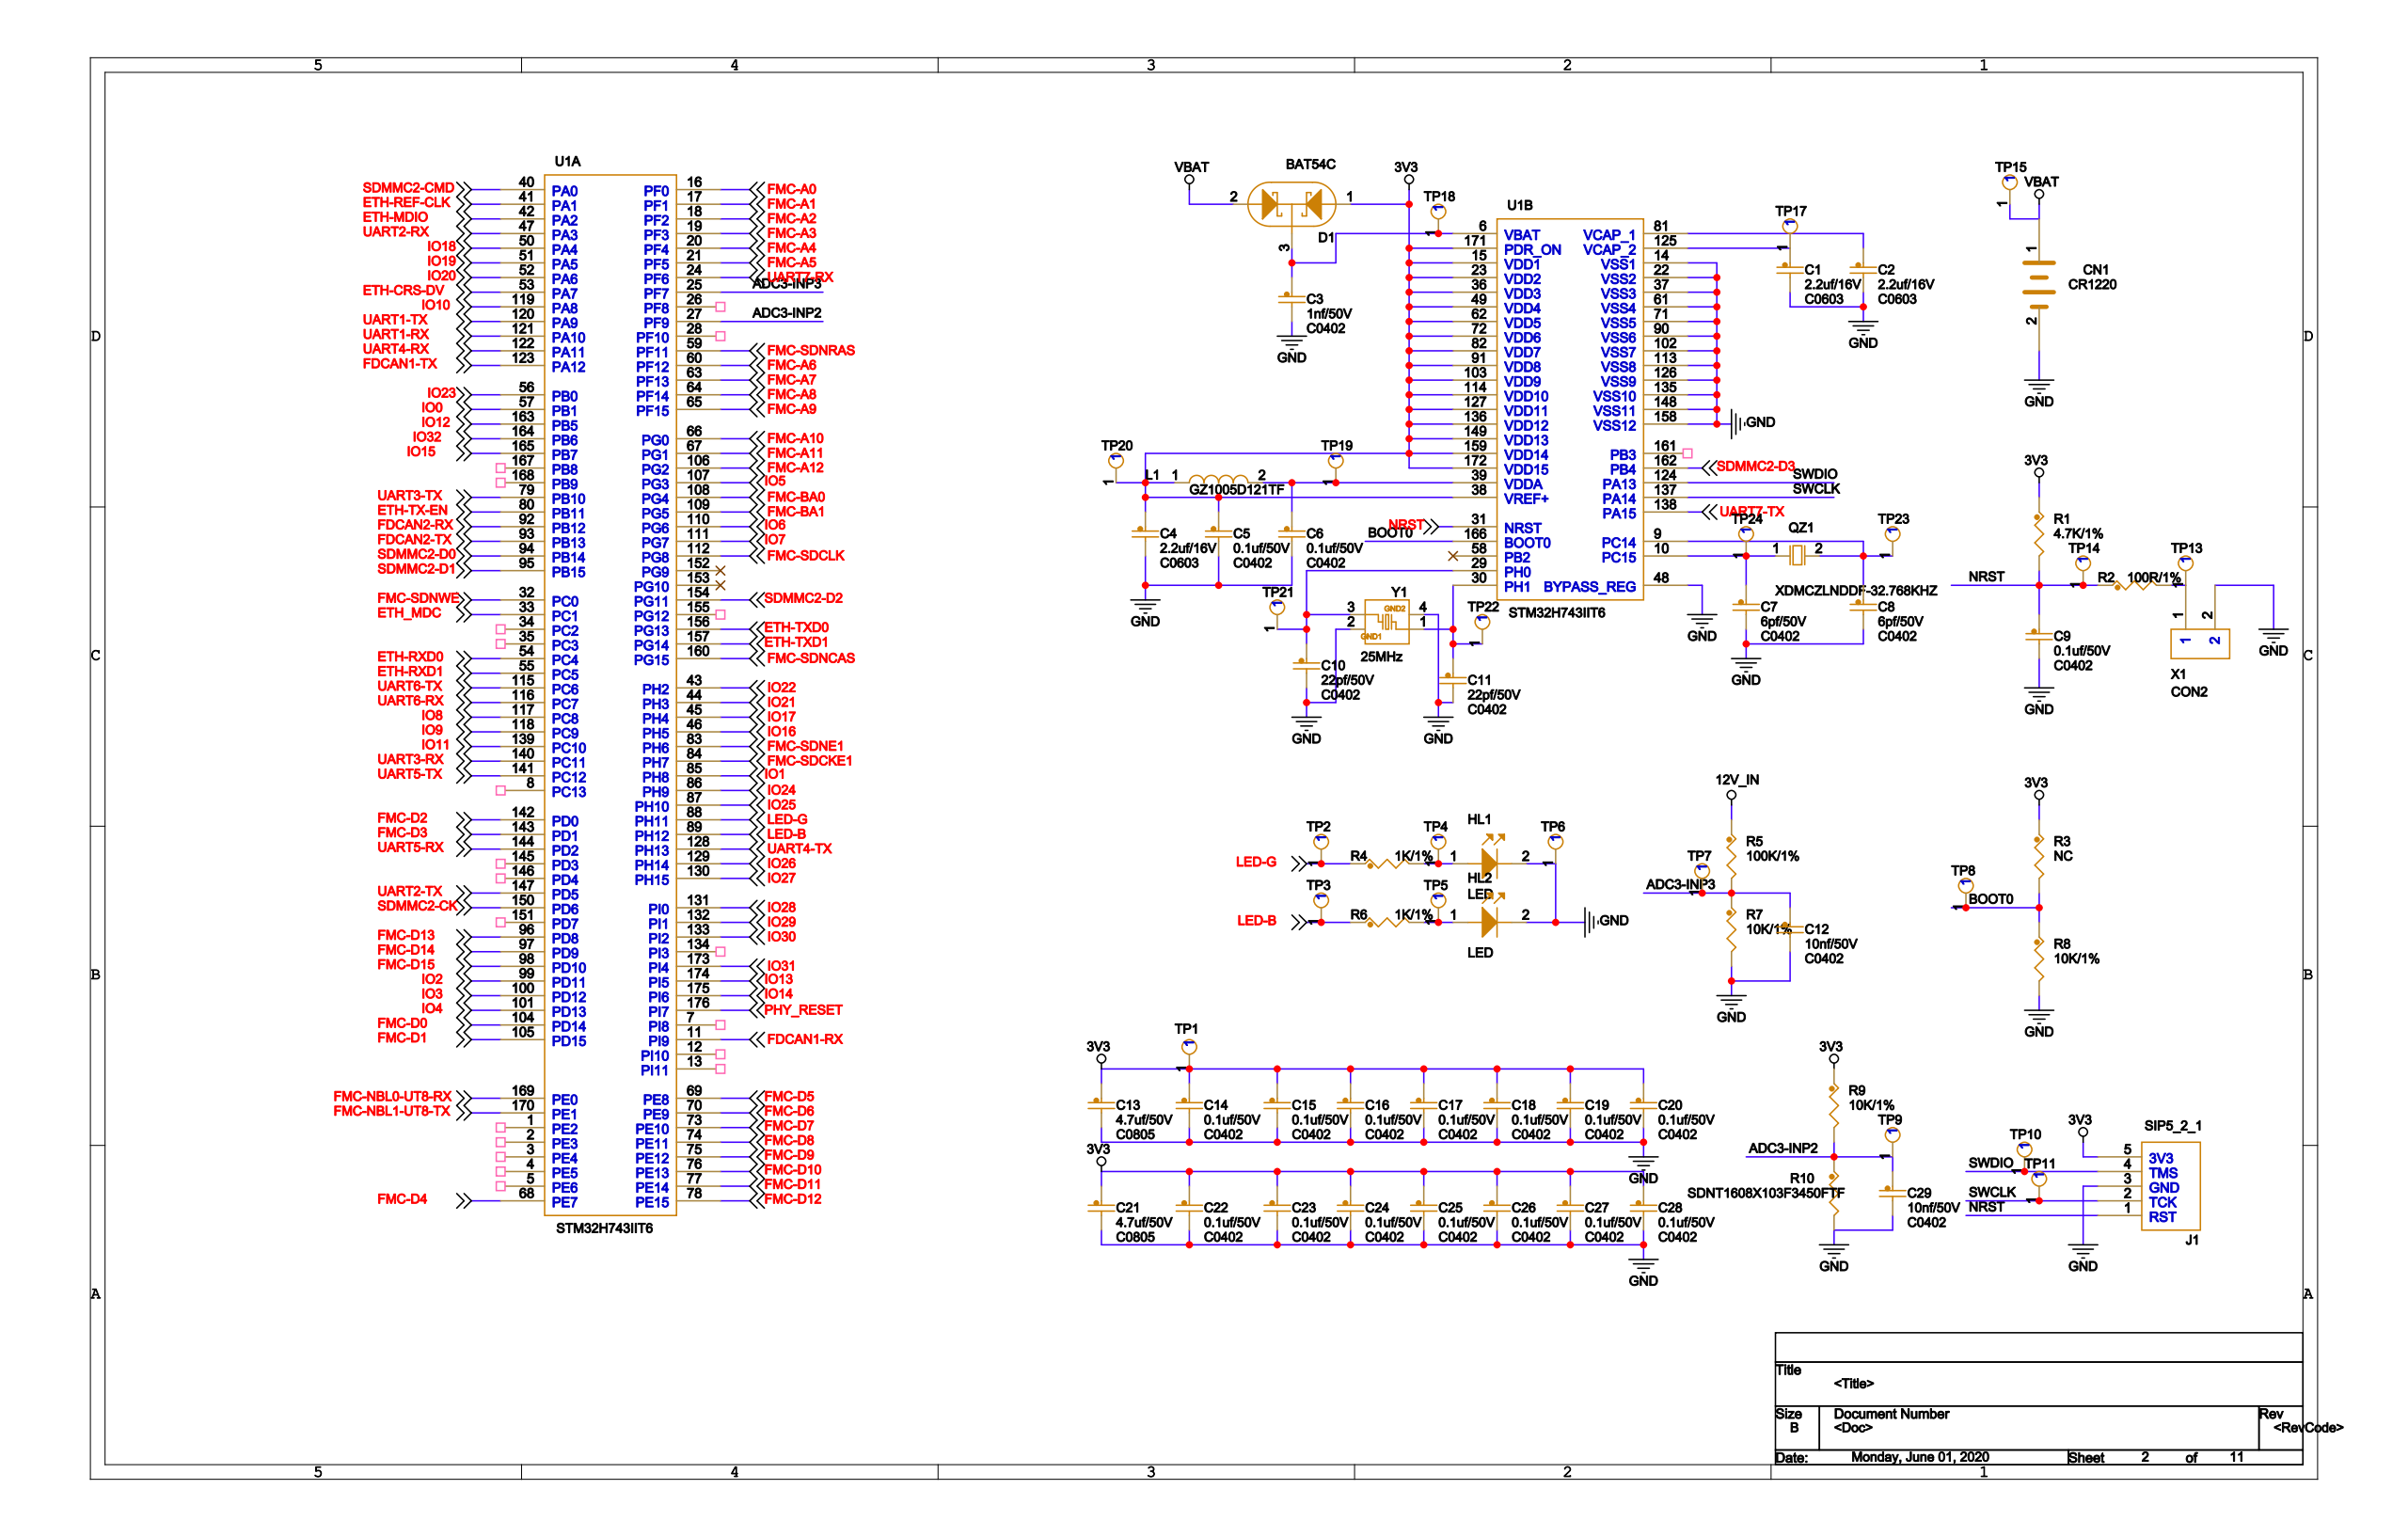Circuit board | Cadence Allegro | 792 parts | 400 nets | one sheet of the schematic
Parts on this sheet (reference | value | footprint):
C1 | 2.2uf/16V | C0603
C2 | 2.2uf/16V | C0603
C3 | 1nf/50V | C0402
C4 | 2.2uf/16V | C0603
C5 | 0.1uf/50V | C0402
C6 | 0.1uf/50V | C0402
C7 | 6pf/50V | C0402
C8 | 6pf/50V | C0402
C9 | 0.1uf/50V | C0402
C10 | 22pf/50V | C0402
C11 | 22pf/50V | C0402
C12 | 10nf/50V | C0402
C13 | 4.7uf/50V | C0805
C14 | 0.1uf/50V | C0402
C15 | 0.1uf/50V | C0402
C16 | 0.1uf/50V | C0402
C17 | 0.1uf/50V | C0402
C18 | 0.1uf/50V | C0402
C19 | 0.1uf/50V | C0402
C20 | 0.1uf/50V | C0402
C21 | 4.7uf/50V | C0805
C22 | 0.1uf/50V | C0402
C23 | 0.1uf/50V | C0402
C24 | 0.1uf/50V | C0402
C25 | 0.1uf/50V | C0402
C26 | 0.1uf/50V | C0402
C27 | 0.1uf/50V | C0402
C28 | 0.1uf/50V | C0402
C29 | 10nf/50V | C0402
CN1 | CR1220 | CR1220
D1 | BAT54C | SOT23
HL1 | LED | LED0603
HL2 | LED | LED0603
J1 | SIP5_2_1 | SIP5
L1 | GZ1005D121TF | 0402
QZ1 | XDMCZLNDDF-32.768KHZ | XTAL_SMD_3215
R1 | 4.7K/1% | 0402
R2 | 100R/1% | 0603
R3 | NC | 0402
R4 | 1K/1% | 0603
R5 | 100K/1% | 0603
R6 | 1K/1% | 0603
R7 | 10K/1% | 0402
R8 | 10K/1% | 0402
R9 | 10K/1% | 0402
R10 | SDNT1608X103F3450FTF | 0603
TP10 | TESTPOINT | TESTPOINT-33MIL
TP11 | TESTPOINT | TESTPOINT-33MIL
TP13 | TESTPOINT | TESTPOINT-33MIL
TP14 | TESTPOINT | TESTPOINT-33MIL
TP15 | TESTPOINT | TESTPOINT-33MIL
TP17 | TESTPOINT | TESTPOINT-33MIL
TP18 | TESTPOINT | TESTPOINT-33MIL
TP19 | TESTPOINT | TESTPOINT-33MIL
TP20 | TESTPOINT | TESTPOINT-33MIL
TP21 | TESTPOINT | TESTPOINT-33MIL
TP22 | TESTPOINT | TESTPOINT-33MIL
TP23 | TESTPOINT | TESTPOINT-33MIL
TP24 | TESTPOINT | TESTPOINT-33MIL
U1 | STM32H743IIT6 | LQFP176
X1 | CON2 | SIP2
Y1 | 25MHz | OSC_SMD3L2X2L5
Nets of these parts (net: part-pin ...):
FMC-NBL0-UT8-RX: U1-169
FMC-NBL1-UT8-TX: U1-170
3V3: C4-1 C5-1 C13-1 C14-1 C15-1 C16-1 C17-1 C18-1 C19-1 C20-1 C21-1 C22-1 C23-1 C24-1 C25-1 C26-1 C27-1 C28-1 D1-1 J1-5 L1-1 R1-1 R3-1 R9-1 TP20-1 U1-15 U1-23 U1-36 U1-38 U1-49 U1-62 U1-72 U1-82 U1-91 U1-103 U1-114 U1-127 U1-136 U1-149 U1-159 U1-171 U1-172
GND: C1-2 C2-2 C3-2 C4-2 C5-2 C6-2 C7-2 C8-2 C9-2 C10-2 C11-2 C12-2 C13-2 C14-2 C15-2 C16-2 C17-2 C18-2 C19-2 C20-2 C21-2 C22-2 C23-2 C24-2 C25-2 C26-2 C27-2 C28-2 C29-2 CN1-2 HL1-2 HL2-2 J1-3 R7-2 R8-2 R10-2 X1-2 Y1-2 Y1-4 U1-14 U1-22 U1-37 U1-48 U1-61 U1-71 U1-90 U1-102 U1-113 U1-126 U1-135 U1-148 U1-158
IO0: U1-57
IO1: U1-85
IO2: U1-99
IO3: U1-100
IO4: U1-101
IO5: U1-107
IO6: U1-110
IO7: U1-111
IO16: U1-46
IO17: U1-45
IO18: U1-50
IO19: U1-51
IO20: U1-52
IO21: U1-44
IO22: U1-43
IO23: U1-56
IO8: U1-117
IO9: U1-118
IO10: U1-119
IO11: U1-139
IO12: U1-163
IO13: U1-174
IO14: U1-175
IO15: U1-165
12V_IN: R5-1
UART5-RX: U1-144
UART5-TX: U1-141
UART2-RX: U1-47
UART2-TX: U1-147
UART6-RX: U1-116
UART6-TX: U1-115
UART7-RX: U1-24
UART7-TX: U1-138
SWDIO: J1-4 TP10-1 U1-124
UART3-RX: U1-140
UART3-TX: U1-79
SWCLK: J1-2 TP11-1 U1-137
UART4-RX: U1-122
UART4-TX: U1-128
N04941: R2-2 TP13-1 X1-1
NRST: C9-1 J1-1 R1-2 R2-1 TP14-1 U1-31
FDCAN2-TX: U1-93
FDCAN2-RX: U1-92
VBAT: CN1-1 D1-2 TP15-1
N05702: C1-1 TP17-1 U1-125
N01856: C3-1 D1-3 TP18-1 U1-6
N02795: C6-1 L1-2 TP19-1 U1-39
LED-G: R4-1 U1-88
N04020: C10-1 TP21-1 Y1-3 U1-29
N04068: C11-1 TP22-1 Y1-1 U1-30
N06443: C8-1 QZ1-2 TP23-1 U1-9
N06439: C7-1 QZ1-1 TP24-1 U1-10
SDMMC2-D2: U1-154
SDMMC2-D3: U1-162
SDMMC2-CMD: U1-40
SDMMC2-CK: U1-150
SDMMC2-D0: U1-94
LED-B: R6-1 U1-89
SDMMC2-D1: U1-95
N7355274: HL1-1 R4-2
PHY_RESET: U1-176
ETH-TX-EN: U1-80
ETH-TXD0: U1-156
ETH-TXD1: U1-157
ETH-RXD1: U1-55
ETH-RXD0: U1-54
ETH-CRS-DV: U1-53
ETH-REF-CLK: U1-41
N7355359: HL2-1 R6-2
ETH_MDC: U1-33
ETH-MDIO: U1-42
ADC3-INP3: C12-1 R5-2 R7-1 U1-25
BOOT0: R3-2 R8-1 U1-166
ADC3-INP2: C29-1 R9-2 R10-1 U1-27
FDCAN1-RX: U1-11
UART1-TX: U1-120
UART1-RX: U1-121
FDCAN1-TX: U1-123
N05695: C2-1 U1-81
IO24: U1-86
IO25: U1-87
IO30: U1-133
IO32: U1-164
IO31: U1-173
IO26: U1-129
IO27: U1-130
IO28: U1-131
IO29: U1-132
FMC-SDNE1: U1-83
FMC-SDNWE: U1-32
FMC-D2: U1-142
FMC-D3: U1-143
FMC-D15: U1-98
FMC-D0: U1-104
FMC-D1: U1-105
FMC-D13: U1-96
FMC-D14: U1-97
FMC-D7: U1-73
FMC-D8: U1-74
FMC-D9: U1-75
FMC-D10: U1-76
FMC-D11: U1-77
FMC-D12: U1-78
FMC-D4: U1-68
FMC-D5: U1-69
FMC-D6: U1-70
FMC-A0: U1-16
FMC-A1: U1-17
FMC-SDNRAS: U1-59
FMC-A6: U1-60
FMC-A7: U1-63
FMC-A8: U1-64
FMC-A9: U1-65
FMC-A2: U1-18
FMC-A3: U1-19
FMC-A4: U1-20
FMC-A5: U1-21
FMC-A10: U1-66
FMC-A11: U1-67
FMC-SDNCAS: U1-160
FMC-A12: U1-106
FMC-BA0: U1-108
FMC-BA1: U1-109
FMC-SDCLK: U1-112
FMC-SDCKE1: U1-84